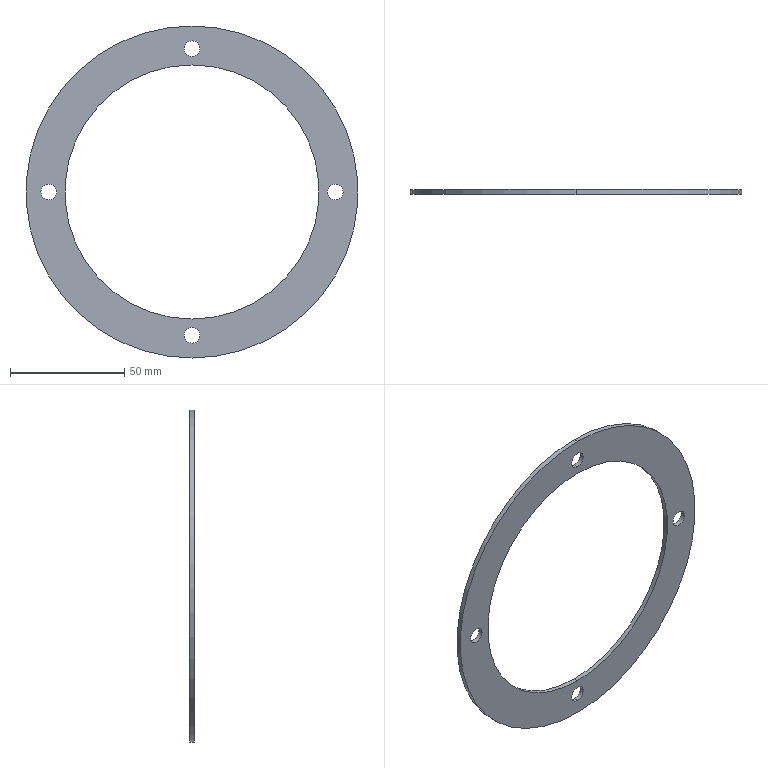Part | SolidWorks | features CirPattern 1, Extrusion 1, ICE 1 | 1 solid | 14 faces | box 145 x 2 x 145 mm | volume 13364 mm3 | cylinder 12 | plane 2 | commonest cylinder face diameters 7 x8 111 x2 145 x2
STEP:
#1=CARTESIAN_POINT('',(66.,0.,0.));
#2=VERTEX_POINT('',#1);
#3=CARTESIAN_POINT('',(59.,0.,0.));
#4=VERTEX_POINT('',#3);
#5=CARTESIAN_POINT('',(62.5,0.,0.));
#6=DIRECTION('',(0.,1.,0.));
#7=DIRECTION('',(-1.,0.,0.));
#8=AXIS2_PLACEMENT_3D('',#5,#6,#7);
#9=CIRCLE('',#8,3.5);
#10=EDGE_CURVE('',#2,#4,#9,.T.);
#11=ORIENTED_EDGE('',*,*,#10,.F.);
#12=CARTESIAN_POINT('',(66.,2.,0.));
#13=VERTEX_POINT('',#12);
#14=CARTESIAN_POINT('',(66.,0.,0.));
#15=DIRECTION('',(0.,1.,0.));
#16=VECTOR('',#15,1000.);
#17=LINE('',#14,#16);
#18=EDGE_CURVE('',#2,#13,#17,.T.);
#19=ORIENTED_EDGE('',*,*,#18,.T.);
#20=CARTESIAN_POINT('',(59.,2.,0.));
#21=VERTEX_POINT('',#20);
#22=CARTESIAN_POINT('',(62.5,2.,0.));
#23=DIRECTION('',(0.,1.,0.));
#24=DIRECTION('',(-1.,0.,0.));
#25=AXIS2_PLACEMENT_3D('',#22,#23,#24);
#26=CIRCLE('',#25,3.5);
#27=EDGE_CURVE('',#13,#21,#26,.T.);
#28=ORIENTED_EDGE('',*,*,#27,.T.);
#29=CARTESIAN_POINT('',(59.,0.,0.));
#30=DIRECTION('',(0.,1.,0.));
#31=VECTOR('',#30,1000.);
#32=LINE('',#29,#31);
#33=EDGE_CURVE('',#4,#21,#32,.T.);
#34=ORIENTED_EDGE('',*,*,#33,.F.);
#35=EDGE_LOOP('',(#11,#19,#28,#34));
#36=FACE_OUTER_BOUND('',#35,.T.);
#37=CARTESIAN_POINT('',(62.5,0.,0.));
#38=DIRECTION('',(0.,1.,0.));
#39=DIRECTION('',(-1.,0.,0.));
#40=AXIS2_PLACEMENT_3D('',#37,#38,#39);
#41=CYLINDRICAL_SURFACE('',#40,3.5);
#42=ADVANCED_FACE('',(#36),#41,.F.);
#43=CARTESIAN_POINT('',(0.,0.,66.));
#44=VERTEX_POINT('',#43);
#45=CARTESIAN_POINT('',(0.,0.,59.));
#46=VERTEX_POINT('',#45);
#47=CARTESIAN_POINT('',(0.,0.,62.5));
#48=DIRECTION('',(0.,1.,0.));
#49=DIRECTION('',(0.,0.,-1.));
#50=AXIS2_PLACEMENT_3D('',#47,#48,#49);
#51=CIRCLE('',#50,3.5);
#52=EDGE_CURVE('',#44,#46,#51,.T.);
#53=ORIENTED_EDGE('',*,*,#52,.F.);
#54=CARTESIAN_POINT('',(0.,2.,66.));
#55=VERTEX_POINT('',#54);
#56=CARTESIAN_POINT('',(0.,0.,66.));
#57=DIRECTION('',(0.,1.,0.));
#58=VECTOR('',#57,1000.);
#59=LINE('',#56,#58);
#60=EDGE_CURVE('',#44,#55,#59,.T.);
#61=ORIENTED_EDGE('',*,*,#60,.T.);
#62=CARTESIAN_POINT('',(0.,2.,59.));
#63=VERTEX_POINT('',#62);
#64=CARTESIAN_POINT('',(0.,2.,62.5));
#65=DIRECTION('',(0.,1.,0.));
#66=DIRECTION('',(0.,0.,-1.));
#67=AXIS2_PLACEMENT_3D('',#64,#65,#66);
#68=CIRCLE('',#67,3.5);
#69=EDGE_CURVE('',#55,#63,#68,.T.);
#70=ORIENTED_EDGE('',*,*,#69,.T.);
#71=CARTESIAN_POINT('',(0.,0.,59.));
#72=DIRECTION('',(0.,1.,0.));
#73=VECTOR('',#72,1000.);
#74=LINE('',#71,#73);
#75=EDGE_CURVE('',#46,#63,#74,.T.);
#76=ORIENTED_EDGE('',*,*,#75,.F.);
#77=EDGE_LOOP('',(#53,#61,#70,#76));
#78=FACE_OUTER_BOUND('',#77,.T.);
#79=CARTESIAN_POINT('',(0.,0.,62.5));
#80=DIRECTION('',(0.,1.,0.));
#81=DIRECTION('',(0.,0.,-1.));
#82=AXIS2_PLACEMENT_3D('',#79,#80,#81);
#83=CYLINDRICAL_SURFACE('',#82,3.5);
#84=ADVANCED_FACE('',(#78),#83,.F.);
#85=CARTESIAN_POINT('',(-66.,0.,0.));
#86=VERTEX_POINT('',#85);
#87=CARTESIAN_POINT('',(-59.,0.,0.));
#88=VERTEX_POINT('',#87);
#89=CARTESIAN_POINT('',(-62.5,0.,0.));
#90=DIRECTION('',(0.,1.,0.));
#91=DIRECTION('',(1.,0.,0.));
#92=AXIS2_PLACEMENT_3D('',#89,#90,#91);
#93=CIRCLE('',#92,3.5);
#94=EDGE_CURVE('',#86,#88,#93,.T.);
#95=ORIENTED_EDGE('',*,*,#94,.F.);
#96=CARTESIAN_POINT('',(-66.,2.,0.));
#97=VERTEX_POINT('',#96);
#98=CARTESIAN_POINT('',(-66.,0.,0.));
#99=DIRECTION('',(0.,1.,0.));
#100=VECTOR('',#99,1000.);
#101=LINE('',#98,#100);
#102=EDGE_CURVE('',#86,#97,#101,.T.);
#103=ORIENTED_EDGE('',*,*,#102,.T.);
#104=CARTESIAN_POINT('',(-59.,2.,0.));
#105=VERTEX_POINT('',#104);
#106=CARTESIAN_POINT('',(-62.5,2.,0.));
#107=DIRECTION('',(0.,1.,0.));
#108=DIRECTION('',(1.,0.,0.));
#109=AXIS2_PLACEMENT_3D('',#106,#107,#108);
#110=CIRCLE('',#109,3.5);
#111=EDGE_CURVE('',#97,#105,#110,.T.);
#112=ORIENTED_EDGE('',*,*,#111,.T.);
#113=CARTESIAN_POINT('',(-59.,0.,0.));
#114=DIRECTION('',(0.,1.,0.));
#115=VECTOR('',#114,1000.);
#116=LINE('',#113,#115);
#117=EDGE_CURVE('',#88,#105,#116,.T.);
#118=ORIENTED_EDGE('',*,*,#117,.F.);
#119=EDGE_LOOP('',(#95,#103,#112,#118));
#120=FACE_OUTER_BOUND('',#119,.T.);
#121=CARTESIAN_POINT('',(-62.5,0.,0.));
#122=DIRECTION('',(0.,1.,0.));
#123=DIRECTION('',(1.,0.,0.));
#124=AXIS2_PLACEMENT_3D('',#121,#122,#123);
#125=CYLINDRICAL_SURFACE('',#124,3.5);
#126=ADVANCED_FACE('',(#120),#125,.F.);
#127=CARTESIAN_POINT('',(0.,0.,-66.));
#128=VERTEX_POINT('',#127);
#129=CARTESIAN_POINT('',(0.,0.,-59.));
#130=VERTEX_POINT('',#129);
#131=CARTESIAN_POINT('',(0.,0.,-62.5));
#132=DIRECTION('',(0.,1.,0.));
#133=DIRECTION('',(0.,0.,1.));
#134=AXIS2_PLACEMENT_3D('',#131,#132,#133);
#135=CIRCLE('',#134,3.5);
#136=EDGE_CURVE('',#128,#130,#135,.T.);
#137=ORIENTED_EDGE('',*,*,#136,.F.);
#138=CARTESIAN_POINT('',(0.,2.,-66.));
#139=VERTEX_POINT('',#138);
#140=CARTESIAN_POINT('',(0.,0.,-66.));
#141=DIRECTION('',(0.,1.,0.));
#142=VECTOR('',#141,1000.);
#143=LINE('',#140,#142);
#144=EDGE_CURVE('',#128,#139,#143,.T.);
#145=ORIENTED_EDGE('',*,*,#144,.T.);
#146=CARTESIAN_POINT('',(0.,2.,-59.));
#147=VERTEX_POINT('',#146);
#148=CARTESIAN_POINT('',(0.,2.,-62.5));
#149=DIRECTION('',(0.,1.,0.));
#150=DIRECTION('',(0.,0.,1.));
#151=AXIS2_PLACEMENT_3D('',#148,#149,#150);
#152=CIRCLE('',#151,3.5);
#153=EDGE_CURVE('',#139,#147,#152,.T.);
#154=ORIENTED_EDGE('',*,*,#153,.T.);
#155=CARTESIAN_POINT('',(0.,0.,-59.));
#156=DIRECTION('',(0.,1.,0.));
#157=VECTOR('',#156,1000.);
#158=LINE('',#155,#157);
#159=EDGE_CURVE('',#130,#147,#158,.T.);
#160=ORIENTED_EDGE('',*,*,#159,.F.);
#161=EDGE_LOOP('',(#137,#145,#154,#160));
#162=FACE_OUTER_BOUND('',#161,.T.);
#163=CARTESIAN_POINT('',(0.,0.,-62.5));
#164=DIRECTION('',(0.,1.,0.));
#165=DIRECTION('',(0.,0.,1.));
#166=AXIS2_PLACEMENT_3D('',#163,#164,#165);
#167=CYLINDRICAL_SURFACE('',#166,3.5);
#168=ADVANCED_FACE('',(#162),#167,.F.);
#169=CARTESIAN_POINT('',(0.,2.,-55.5));
#170=VERTEX_POINT('',#169);
#171=CARTESIAN_POINT('',(0.,2.,55.5));
#172=VERTEX_POINT('',#171);
#173=CARTESIAN_POINT('',(0.,2.,0.));
#174=DIRECTION('',(0.,1.,0.));
#175=DIRECTION('',(0.,0.,1.));
#176=AXIS2_PLACEMENT_3D('',#173,#174,#175);
#177=CIRCLE('',#176,55.5);
#178=EDGE_CURVE('',#170,#172,#177,.T.);
#179=ORIENTED_EDGE('',*,*,#178,.T.);
#180=CARTESIAN_POINT('',(0.,0.,55.5));
#181=VERTEX_POINT('',#180);
#182=CARTESIAN_POINT('',(0.,2.,55.5));
#183=DIRECTION('',(0.,-1.,0.));
#184=VECTOR('',#183,1000.);
#185=LINE('',#182,#184);
#186=EDGE_CURVE('',#172,#181,#185,.T.);
#187=ORIENTED_EDGE('',*,*,#186,.T.);
#188=CARTESIAN_POINT('',(0.,0.,-55.5));
#189=VERTEX_POINT('',#188);
#190=CARTESIAN_POINT('',(0.,0.,0.));
#191=DIRECTION('',(0.,1.,0.));
#192=DIRECTION('',(0.,0.,1.));
#193=AXIS2_PLACEMENT_3D('',#190,#191,#192);
#194=CIRCLE('',#193,55.5);
#195=EDGE_CURVE('',#189,#181,#194,.T.);
#196=ORIENTED_EDGE('',*,*,#195,.F.);
#197=CARTESIAN_POINT('',(0.,2.,-55.5));
#198=DIRECTION('',(0.,-1.,0.));
#199=VECTOR('',#198,1000.);
#200=LINE('',#197,#199);
#201=EDGE_CURVE('',#170,#189,#200,.T.);
#202=ORIENTED_EDGE('',*,*,#201,.F.);
#203=EDGE_LOOP('',(#179,#187,#196,#202));
#204=FACE_OUTER_BOUND('',#203,.T.);
#205=CARTESIAN_POINT('',(0.,2.,0.));
#206=DIRECTION('',(0.,-1.,0.));
#207=DIRECTION('',(0.,0.,-1.));
#208=AXIS2_PLACEMENT_3D('',#205,#206,#207);
#209=CYLINDRICAL_SURFACE('',#208,55.5);
#210=ADVANCED_FACE('',(#204),#209,.F.);
#211=CARTESIAN_POINT('',(0.,2.,72.5));
#212=VERTEX_POINT('',#211);
#213=CARTESIAN_POINT('',(0.,2.,-72.5));
#214=VERTEX_POINT('',#213);
#215=CARTESIAN_POINT('',(0.,2.,0.));
#216=DIRECTION('',(0.,1.,0.));
#217=DIRECTION('',(0.,0.,1.));
#218=AXIS2_PLACEMENT_3D('',#215,#216,#217);
#219=CIRCLE('',#218,72.5);
#220=EDGE_CURVE('',#212,#214,#219,.T.);
#221=ORIENTED_EDGE('',*,*,#220,.F.);
#222=CARTESIAN_POINT('',(0.,0.,72.5));
#223=VERTEX_POINT('',#222);
#224=CARTESIAN_POINT('',(0.,2.,72.5));
#225=DIRECTION('',(0.,-1.,0.));
#226=VECTOR('',#225,1000.);
#227=LINE('',#224,#226);
#228=EDGE_CURVE('',#212,#223,#227,.T.);
#229=ORIENTED_EDGE('',*,*,#228,.T.);
#230=CARTESIAN_POINT('',(0.,0.,-72.5));
#231=VERTEX_POINT('',#230);
#232=CARTESIAN_POINT('',(0.,0.,0.));
#233=DIRECTION('',(0.,1.,0.));
#234=DIRECTION('',(0.,0.,1.));
#235=AXIS2_PLACEMENT_3D('',#232,#233,#234);
#236=CIRCLE('',#235,72.5);
#237=EDGE_CURVE('',#223,#231,#236,.T.);
#238=ORIENTED_EDGE('',*,*,#237,.T.);
#239=CARTESIAN_POINT('',(0.,2.,-72.5));
#240=DIRECTION('',(0.,-1.,0.));
#241=VECTOR('',#240,1000.);
#242=LINE('',#239,#241);
#243=EDGE_CURVE('',#214,#231,#242,.T.);
#244=ORIENTED_EDGE('',*,*,#243,.F.);
#245=EDGE_LOOP('',(#221,#229,#238,#244));
#246=FACE_OUTER_BOUND('',#245,.T.);
#247=CARTESIAN_POINT('',(0.,2.,0.));
#248=DIRECTION('',(0.,-1.,0.));
#249=DIRECTION('',(0.,0.,-1.));
#250=AXIS2_PLACEMENT_3D('',#247,#248,#249);
#251=CYLINDRICAL_SURFACE('',#250,72.5);
#252=ADVANCED_FACE('',(#246),#251,.T.);
#253=CARTESIAN_POINT('',(62.5,2.,0.));
#254=DIRECTION('',(0.,1.,0.));
#255=DIRECTION('',(-1.,0.,0.));
#256=AXIS2_PLACEMENT_3D('',#253,#254,#255);
#257=CIRCLE('',#256,3.5);
#258=EDGE_CURVE('',#21,#13,#257,.T.);
#259=ORIENTED_EDGE('',*,*,#258,.F.);
#260=ORIENTED_EDGE('',*,*,#27,.F.);
#261=EDGE_LOOP('',(#259,#260));
#262=FACE_BOUND('',#261,.T.);
#263=CARTESIAN_POINT('',(0.,2.,62.5));
#264=DIRECTION('',(0.,1.,0.));
#265=DIRECTION('',(0.,0.,-1.));
#266=AXIS2_PLACEMENT_3D('',#263,#264,#265);
#267=CIRCLE('',#266,3.5);
#268=EDGE_CURVE('',#63,#55,#267,.T.);
#269=ORIENTED_EDGE('',*,*,#268,.F.);
#270=ORIENTED_EDGE('',*,*,#69,.F.);
#271=EDGE_LOOP('',(#269,#270));
#272=FACE_BOUND('',#271,.T.);
#273=CARTESIAN_POINT('',(-62.5,2.,0.));
#274=DIRECTION('',(0.,1.,0.));
#275=DIRECTION('',(1.,0.,0.));
#276=AXIS2_PLACEMENT_3D('',#273,#274,#275);
#277=CIRCLE('',#276,3.5);
#278=EDGE_CURVE('',#105,#97,#277,.T.);
#279=ORIENTED_EDGE('',*,*,#278,.F.);
#280=ORIENTED_EDGE('',*,*,#111,.F.);
#281=EDGE_LOOP('',(#279,#280));
#282=FACE_BOUND('',#281,.T.);
#283=CARTESIAN_POINT('',(0.,2.,-62.5));
#284=DIRECTION('',(0.,1.,0.));
#285=DIRECTION('',(0.,0.,1.));
#286=AXIS2_PLACEMENT_3D('',#283,#284,#285);
#287=CIRCLE('',#286,3.5);
#288=EDGE_CURVE('',#147,#139,#287,.T.);
#289=ORIENTED_EDGE('',*,*,#288,.F.);
#290=ORIENTED_EDGE('',*,*,#153,.F.);
#291=EDGE_LOOP('',(#289,#290));
#292=FACE_BOUND('',#291,.T.);
#293=CARTESIAN_POINT('',(0.,2.,0.));
#294=DIRECTION('',(0.,1.,0.));
#295=DIRECTION('',(0.,0.,1.));
#296=AXIS2_PLACEMENT_3D('',#293,#294,#295);
#297=CIRCLE('',#296,72.5);
#298=EDGE_CURVE('',#214,#212,#297,.T.);
#299=ORIENTED_EDGE('',*,*,#298,.T.);
#300=ORIENTED_EDGE('',*,*,#220,.T.);
#301=EDGE_LOOP('',(#299,#300));
#302=FACE_OUTER_BOUND('',#301,.T.);
#303=ORIENTED_EDGE('',*,*,#178,.F.);
#304=CARTESIAN_POINT('',(0.,2.,0.));
#305=DIRECTION('',(0.,1.,0.));
#306=DIRECTION('',(0.,0.,1.));
#307=AXIS2_PLACEMENT_3D('',#304,#305,#306);
#308=CIRCLE('',#307,55.5);
#309=EDGE_CURVE('',#172,#170,#308,.T.);
#310=ORIENTED_EDGE('',*,*,#309,.F.);
#311=EDGE_LOOP('',(#303,#310));
#312=FACE_BOUND('',#311,.T.);
#313=CARTESIAN_POINT('',(0.,2.,0.));
#314=DIRECTION('',(0.,1.,0.));
#315=DIRECTION('',(0.,0.,1.));
#316=AXIS2_PLACEMENT_3D('',#313,#314,#315);
#317=PLANE('',#316);
#318=ADVANCED_FACE('',(#262,#272,#282,#292,#302,#312),#317,.T.);
#319=CARTESIAN_POINT('',(62.5,0.,0.));
#320=DIRECTION('',(0.,1.,0.));
#321=DIRECTION('',(-1.,0.,0.));
#322=AXIS2_PLACEMENT_3D('',#319,#320,#321);
#323=CIRCLE('',#322,3.5);
#324=EDGE_CURVE('',#4,#2,#323,.T.);
#325=ORIENTED_EDGE('',*,*,#324,.T.);
#326=ORIENTED_EDGE('',*,*,#10,.T.);
#327=EDGE_LOOP('',(#325,#326));
#328=FACE_BOUND('',#327,.T.);
#329=CARTESIAN_POINT('',(0.,0.,62.5));
#330=DIRECTION('',(0.,1.,0.));
#331=DIRECTION('',(0.,0.,-1.));
#332=AXIS2_PLACEMENT_3D('',#329,#330,#331);
#333=CIRCLE('',#332,3.5);
#334=EDGE_CURVE('',#46,#44,#333,.T.);
#335=ORIENTED_EDGE('',*,*,#334,.T.);
#336=ORIENTED_EDGE('',*,*,#52,.T.);
#337=EDGE_LOOP('',(#335,#336));
#338=FACE_BOUND('',#337,.T.);
#339=CARTESIAN_POINT('',(-62.5,0.,0.));
#340=DIRECTION('',(0.,1.,0.));
#341=DIRECTION('',(1.,0.,0.));
#342=AXIS2_PLACEMENT_3D('',#339,#340,#341);
#343=CIRCLE('',#342,3.5);
#344=EDGE_CURVE('',#88,#86,#343,.T.);
#345=ORIENTED_EDGE('',*,*,#344,.T.);
#346=ORIENTED_EDGE('',*,*,#94,.T.);
#347=EDGE_LOOP('',(#345,#346));
#348=FACE_BOUND('',#347,.T.);
#349=CARTESIAN_POINT('',(0.,0.,-62.5));
#350=DIRECTION('',(0.,1.,0.));
#351=DIRECTION('',(0.,0.,1.));
#352=AXIS2_PLACEMENT_3D('',#349,#350,#351);
#353=CIRCLE('',#352,3.5);
#354=EDGE_CURVE('',#130,#128,#353,.T.);
#355=ORIENTED_EDGE('',*,*,#354,.T.);
#356=ORIENTED_EDGE('',*,*,#136,.T.);
#357=EDGE_LOOP('',(#355,#356));
#358=FACE_BOUND('',#357,.T.);
#359=CARTESIAN_POINT('',(0.,0.,0.));
#360=DIRECTION('',(0.,1.,0.));
#361=DIRECTION('',(0.,0.,1.));
#362=AXIS2_PLACEMENT_3D('',#359,#360,#361);
#363=CIRCLE('',#362,72.5);
#364=EDGE_CURVE('',#231,#223,#363,.T.);
#365=ORIENTED_EDGE('',*,*,#364,.F.);
#366=ORIENTED_EDGE('',*,*,#237,.F.);
#367=EDGE_LOOP('',(#365,#366));
#368=FACE_OUTER_BOUND('',#367,.T.);
#369=ORIENTED_EDGE('',*,*,#195,.T.);
#370=CARTESIAN_POINT('',(0.,0.,0.));
#371=DIRECTION('',(0.,1.,0.));
#372=DIRECTION('',(0.,0.,1.));
#373=AXIS2_PLACEMENT_3D('',#370,#371,#372);
#374=CIRCLE('',#373,55.5);
#375=EDGE_CURVE('',#181,#189,#374,.T.);
#376=ORIENTED_EDGE('',*,*,#375,.T.);
#377=EDGE_LOOP('',(#369,#376));
#378=FACE_BOUND('',#377,.T.);
#379=CARTESIAN_POINT('',(0.,0.,0.));
#380=DIRECTION('',(0.,1.,0.));
#381=DIRECTION('',(0.,0.,1.));
#382=AXIS2_PLACEMENT_3D('',#379,#380,#381);
#383=PLANE('',#382);
#384=ADVANCED_FACE('',(#328,#338,#348,#358,#368,#378),#383,.F.);
#385=ORIENTED_EDGE('',*,*,#228,.F.);
#386=ORIENTED_EDGE('',*,*,#298,.F.);
#387=ORIENTED_EDGE('',*,*,#243,.T.);
#388=ORIENTED_EDGE('',*,*,#364,.T.);
#389=EDGE_LOOP('',(#385,#386,#387,#388));
#390=FACE_OUTER_BOUND('',#389,.T.);
#391=CARTESIAN_POINT('',(0.,2.,0.));
#392=DIRECTION('',(0.,-1.,0.));
#393=DIRECTION('',(0.,0.,-1.));
#394=AXIS2_PLACEMENT_3D('',#391,#392,#393);
#395=CYLINDRICAL_SURFACE('',#394,72.5);
#396=ADVANCED_FACE('',(#390),#395,.T.);
#397=ORIENTED_EDGE('',*,*,#186,.F.);
#398=ORIENTED_EDGE('',*,*,#309,.T.);
#399=ORIENTED_EDGE('',*,*,#201,.T.);
#400=ORIENTED_EDGE('',*,*,#375,.F.);
#401=EDGE_LOOP('',(#397,#398,#399,#400));
#402=FACE_OUTER_BOUND('',#401,.T.);
#403=CARTESIAN_POINT('',(0.,2.,0.));
#404=DIRECTION('',(0.,-1.,0.));
#405=DIRECTION('',(0.,0.,-1.));
#406=AXIS2_PLACEMENT_3D('',#403,#404,#405);
#407=CYLINDRICAL_SURFACE('',#406,55.5);
#408=ADVANCED_FACE('',(#402),#407,.F.);
#409=ORIENTED_EDGE('',*,*,#144,.F.);
#410=ORIENTED_EDGE('',*,*,#354,.F.);
#411=ORIENTED_EDGE('',*,*,#159,.T.);
#412=ORIENTED_EDGE('',*,*,#288,.T.);
#413=EDGE_LOOP('',(#409,#410,#411,#412));
#414=FACE_OUTER_BOUND('',#413,.T.);
#415=CARTESIAN_POINT('',(0.,0.,-62.5));
#416=DIRECTION('',(0.,1.,0.));
#417=DIRECTION('',(0.,0.,1.));
#418=AXIS2_PLACEMENT_3D('',#415,#416,#417);
#419=CYLINDRICAL_SURFACE('',#418,3.5);
#420=ADVANCED_FACE('',(#414),#419,.F.);
#421=ORIENTED_EDGE('',*,*,#102,.F.);
#422=ORIENTED_EDGE('',*,*,#344,.F.);
#423=ORIENTED_EDGE('',*,*,#117,.T.);
#424=ORIENTED_EDGE('',*,*,#278,.T.);
#425=EDGE_LOOP('',(#421,#422,#423,#424));
#426=FACE_OUTER_BOUND('',#425,.T.);
#427=CARTESIAN_POINT('',(-62.5,0.,0.));
#428=DIRECTION('',(0.,1.,0.));
#429=DIRECTION('',(1.,0.,0.));
#430=AXIS2_PLACEMENT_3D('',#427,#428,#429);
#431=CYLINDRICAL_SURFACE('',#430,3.5);
#432=ADVANCED_FACE('',(#426),#431,.F.);
#433=ORIENTED_EDGE('',*,*,#60,.F.);
#434=ORIENTED_EDGE('',*,*,#334,.F.);
#435=ORIENTED_EDGE('',*,*,#75,.T.);
#436=ORIENTED_EDGE('',*,*,#268,.T.);
#437=EDGE_LOOP('',(#433,#434,#435,#436));
#438=FACE_OUTER_BOUND('',#437,.T.);
#439=CARTESIAN_POINT('',(0.,0.,62.5));
#440=DIRECTION('',(0.,1.,0.));
#441=DIRECTION('',(0.,0.,-1.));
#442=AXIS2_PLACEMENT_3D('',#439,#440,#441);
#443=CYLINDRICAL_SURFACE('',#442,3.5);
#444=ADVANCED_FACE('',(#438),#443,.F.);
#445=ORIENTED_EDGE('',*,*,#18,.F.);
#446=ORIENTED_EDGE('',*,*,#324,.F.);
#447=ORIENTED_EDGE('',*,*,#33,.T.);
#448=ORIENTED_EDGE('',*,*,#258,.T.);
#449=EDGE_LOOP('',(#445,#446,#447,#448));
#450=FACE_OUTER_BOUND('',#449,.T.);
#451=CARTESIAN_POINT('',(62.5,0.,0.));
#452=DIRECTION('',(0.,1.,0.));
#453=DIRECTION('',(-1.,0.,0.));
#454=AXIS2_PLACEMENT_3D('',#451,#452,#453);
#455=CYLINDRICAL_SURFACE('',#454,3.5);
#456=ADVANCED_FACE('',(#450),#455,.F.);
#457=CLOSED_SHELL('',(#42,#84,#126,#168,#210,#252,#318,#384,#396,#408,#420,#432,#444,#456));
#458=MANIFOLD_SOLID_BREP('',#457);
#459=CARTESIAN_POINT('',(0.,0.,0.));
#460=DIRECTION('',(0.,0.,1.));
#461=DIRECTION('',(1.,0.,0.));
#462=AXIS2_PLACEMENT_3D('',#459,#460,#461);
#463=(LENGTH_UNIT()NAMED_UNIT(*)SI_UNIT(.MILLI.,.METRE.));
#464=UNCERTAINTY_MEASURE_WITH_UNIT(LENGTH_MEASURE(0.00001),#463,'','');
#465=(NAMED_UNIT(*)PLANE_ANGLE_UNIT()SI_UNIT($,.RADIAN.));
#466=(NAMED_UNIT(*)SI_UNIT($,.STERADIAN.)SOLID_ANGLE_UNIT());
#467=(GEOMETRIC_REPRESENTATION_CONTEXT(3)GLOBAL_UNCERTAINTY_ASSIGNED_CONTEXT((#464))GLOBAL_UNIT_ASSIGNED_CONTEXT((#463,#465,#466))REPRESENTATION_CONTEXT('',''));
#468=ADVANCED_BREP_SHAPE_REPRESENTATION('',(#458,#462),#467);